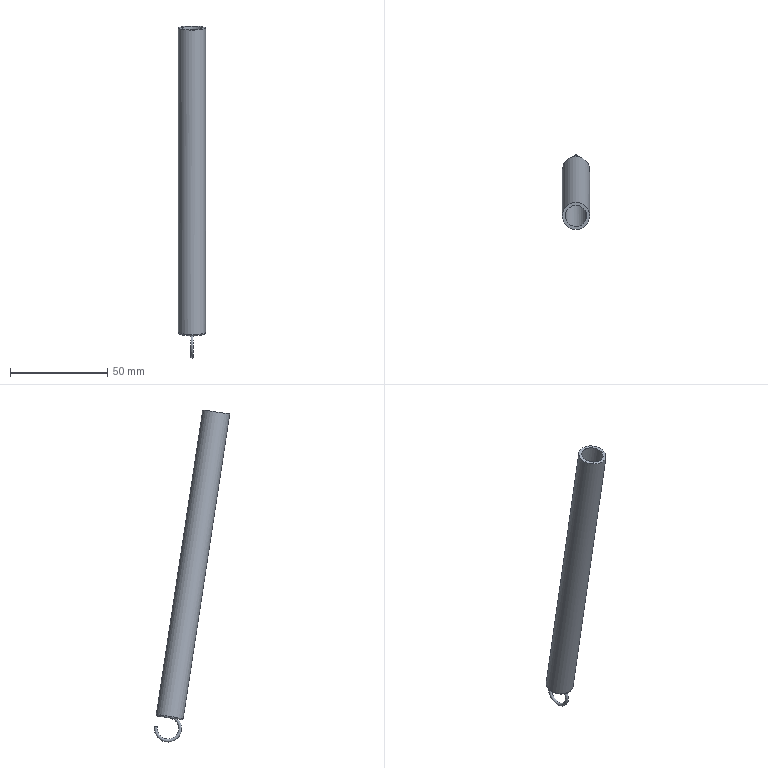Part | NX | features solid 2 | 1 solid | 7 faces | box 14 x 38.697 x 170.602 mm | volume 9414 mm3 | cylinder 3 | torus 2 | plane 2 | commonest cylinder face diameters 1.5 x1 11 x1 14 x1
STEP:
#1=CARTESIAN_POINT('',(-31.935,95.659,-933.338));
#2=VERTEX_POINT('',#1);
#3=CARTESIAN_POINT('',(-24.935,95.659,-933.338));
#4=DIRECTION('',(0.,-0.1507,0.9886));
#5=DIRECTION('',(-1.,0.,0.));
#6=AXIS2_PLACEMENT_3D('',#3,#4,#5);
#7=CIRCLE('',#6,7.);
#8=EDGE_CURVE('',#2,#2,#7,.T.);
#9=ORIENTED_EDGE('',*,*,#8,.T.);
#10=EDGE_LOOP('',(#9));
#11=FACE_BOUND('',#10,.T.);
#12=CARTESIAN_POINT('',(-24.935,78.749,-775.915));
#13=VERTEX_POINT('',#12);
#14=CARTESIAN_POINT('',(-24.935,71.827,-776.952));
#15=DIRECTION('',(0.,-0.1481,0.989));
#16=DIRECTION('',(0.,0.989,0.1481));
#17=AXIS2_PLACEMENT_3D('',#14,#15,#16);
#18=ELLIPSE('',#17,7.,7.);
#19=EDGE_CURVE('',#13,#13,#18,.F.);
#20=ORIENTED_EDGE('',*,*,#19,.T.);
#21=EDGE_LOOP('',(#20));
#22=FACE_BOUND('',#21,.T.);
#23=CARTESIAN_POINT('',(-24.935,59.467,-695.849));
#24=DIRECTION('',(0.,0.1507,-0.9886));
#25=DIRECTION('',(1.,0.,0.));
#26=AXIS2_PLACEMENT_3D('',#23,#24,#25);
#27=CYLINDRICAL_SURFACE('',#26,7.);
#28=ADVANCED_FACE('',(#11,#22),#27,.T.);
#29=CARTESIAN_POINT('',(-25.685,101.046,-932.517));
#30=VERTEX_POINT('',#29);
#31=CARTESIAN_POINT('',(-24.185,101.046,-932.517));
#32=VERTEX_POINT('',#31);
#33=CARTESIAN_POINT('',(-24.935,95.659,-933.338));
#34=DIRECTION('',(0.,-0.1507,0.9886));
#35=DIRECTION('',(1.,0.,0.));
#36=AXIS2_PLACEMENT_3D('',#33,#34,#35);
#37=CIRCLE('',#36,5.5);
#38=EDGE_CURVE('',#30,#32,#37,.T.);
#39=ORIENTED_EDGE('',*,*,#38,.F.);
#40=CARTESIAN_POINT('',(-24.185,101.046,-932.517));
#41=CARTESIAN_POINT('',(-24.185,100.986,-932.125));
#42=CARTESIAN_POINT('',(-24.934,100.981,-931.411));
#43=CARTESIAN_POINT('',(-25.685,100.986,-932.125));
#44=CARTESIAN_POINT('',(-25.685,101.046,-932.517));
#45=B_SPLINE_CURVE_WITH_KNOTS('',3,(#40,#41,#42,#43,#44),.UNSPECIFIED.,.F.,.F.,(4,1,4),(0.,0.001174,0.002347),.UNSPECIFIED.);
#46=EDGE_CURVE('',#32,#30,#45,.T.);
#47=ORIENTED_EDGE('',*,*,#46,.F.);
#48=EDGE_LOOP('',(#39,#47));
#49=FACE_BOUND('',#48,.T.);
#50=CARTESIAN_POINT('',(-24.935,77.266,-776.137));
#51=VERTEX_POINT('',#50);
#52=CARTESIAN_POINT('',(-24.935,71.827,-776.952));
#53=DIRECTION('',(0.,-0.1481,0.989));
#54=DIRECTION('',(0.,0.989,0.1481));
#55=AXIS2_PLACEMENT_3D('',#52,#53,#54);
#56=ELLIPSE('',#55,5.5,5.5);
#57=EDGE_CURVE('',#51,#51,#56,.T.);
#58=ORIENTED_EDGE('',*,*,#57,.T.);
#59=EDGE_LOOP('',(#58));
#60=FACE_BOUND('',#59,.T.);
#61=CARTESIAN_POINT('',(-24.935,59.467,-695.849));
#62=DIRECTION('',(0.,0.1507,-0.9886));
#63=DIRECTION('',(1.,0.,0.));
#64=AXIS2_PLACEMENT_3D('',#61,#62,#63);
#65=CYLINDRICAL_SURFACE('',#64,5.5);
#66=ADVANCED_FACE('',(#49,#60),#65,.F.);
#67=ORIENTED_EDGE('',*,*,#38,.T.);
#68=CARTESIAN_POINT('',(-24.935,101.951,-933.138));
#69=VERTEX_POINT('',#68);
#70=CARTESIAN_POINT('',(-24.185,101.046,-932.517));
#71=CARTESIAN_POINT('',(-24.185,101.083,-932.761));
#72=CARTESIAN_POINT('',(-24.428,101.419,-933.116));
#73=CARTESIAN_POINT('',(-24.763,101.781,-933.164));
#74=CARTESIAN_POINT('',(-24.935,101.951,-933.138));
#75=B_SPLINE_CURVE_WITH_KNOTS('',3,(#70,#71,#72,#73,#74),.UNSPECIFIED.,.F.,.F.,(4,1,4),(0.,0.0007272,0.001454),.UNSPECIFIED.);
#76=EDGE_CURVE('',#32,#69,#75,.T.);
#77=ORIENTED_EDGE('',*,*,#76,.T.);
#78=CARTESIAN_POINT('',(-25.685,101.046,-932.517));
#79=CARTESIAN_POINT('',(-25.685,101.083,-932.761));
#80=CARTESIAN_POINT('',(-25.442,101.419,-933.116));
#81=CARTESIAN_POINT('',(-25.106,101.781,-933.164));
#82=CARTESIAN_POINT('',(-24.935,101.951,-933.138));
#83=B_SPLINE_CURVE_WITH_KNOTS('',3,(#78,#79,#80,#81,#82),.UNSPECIFIED.,.F.,.F.,(4,1,4),(0.,0.0007272,0.001454),.UNSPECIFIED.);
#84=EDGE_CURVE('',#69,#30,#83,.F.);
#85=ORIENTED_EDGE('',*,*,#84,.T.);
#86=EDGE_LOOP('',(#67,#77,#85));
#87=FACE_BOUND('',#86,.T.);
#88=ORIENTED_EDGE('',*,*,#8,.F.);
#89=EDGE_LOOP('',(#88));
#90=FACE_BOUND('',#89,.T.);
#91=CARTESIAN_POINT('',(-24.935,95.659,-933.338));
#92=DIRECTION('',(0.,-0.1507,0.9886));
#93=DIRECTION('',(1.,0.,0.));
#94=AXIS2_PLACEMENT_3D('',#91,#92,#93);
#95=TOROIDAL_SURFACE('',#94,6.25,0.75);
#96=ADVANCED_FACE('',(#87,#90),#95,.T.);
#97=CARTESIAN_POINT('',(-24.935,103.501,-938.342));
#98=VERTEX_POINT('',#97);
#99=CARTESIAN_POINT('',(-24.935,102.762,-938.468));
#100=DIRECTION('',(0.,0.1679,-0.9858));
#101=DIRECTION('',(0.,0.9858,0.1679));
#102=AXIS2_PLACEMENT_3D('',#99,#100,#101);
#103=CIRCLE('',#102,0.75);
#104=EDGE_CURVE('',#98,#98,#103,.T.);
#105=ORIENTED_EDGE('',*,*,#104,.T.);
#106=EDGE_LOOP('',(#105));
#107=FACE_BOUND('',#106,.T.);
#108=CARTESIAN_POINT('',(-25.685,95.659,-933.338));
#109=VERTEX_POINT('',#108);
#110=CARTESIAN_POINT('',(-24.935,95.659,-933.338));
#111=DIRECTION('',(0.,0.9886,0.1507));
#112=DIRECTION('',(-1.,0.,0.));
#113=AXIS2_PLACEMENT_3D('',#110,#111,#112);
#114=CIRCLE('',#113,0.75);
#115=EDGE_CURVE('',#109,#109,#114,.T.);
#116=ORIENTED_EDGE('',*,*,#115,.F.);
#117=EDGE_LOOP('',(#116));
#118=FACE_BOUND('',#117,.T.);
#119=CARTESIAN_POINT('',(-24.935,96.601,-939.517));
#120=DIRECTION('',(1.,0.,0.));
#121=DIRECTION('',(0.,0.1507,-0.9886));
#122=AXIS2_PLACEMENT_3D('',#119,#120,#121);
#123=TOROIDAL_SURFACE('',#122,6.25,0.75);
#124=ADVANCED_FACE('',(#107,#118),#123,.T.);
#125=ORIENTED_EDGE('',*,*,#115,.T.);
#126=EDGE_LOOP('',(#125));
#127=FACE_BOUND('',#126,.T.);
#128=ORIENTED_EDGE('',*,*,#76,.F.);
#129=ORIENTED_EDGE('',*,*,#46,.T.);
#130=ORIENTED_EDGE('',*,*,#84,.F.);
#131=EDGE_LOOP('',(#128,#129,#130));
#132=FACE_BOUND('',#131,.T.);
#133=CARTESIAN_POINT('',(-24.935,98.748,-932.867));
#134=DIRECTION('',(0.,-0.9886,-0.1507));
#135=DIRECTION('',(1.,0.,0.));
#136=AXIS2_PLACEMENT_3D('',#133,#134,#135);
#137=CYLINDRICAL_SURFACE('',#136,0.75);
#138=ADVANCED_FACE('',(#127,#132),#137,.T.);
#139=ORIENTED_EDGE('',*,*,#104,.F.);
#140=EDGE_LOOP('',(#139));
#141=FACE_BOUND('',#140,.T.);
#142=CARTESIAN_POINT('',(-24.935,102.762,-938.468));
#143=DIRECTION('',(0.,0.1679,-0.9858));
#144=DIRECTION('',(0.,-0.9858,-0.1679));
#145=AXIS2_PLACEMENT_3D('',#142,#143,#144);
#146=PLANE('',#145);
#147=ADVANCED_FACE('',(#141),#146,.F.);
#148=ORIENTED_EDGE('',*,*,#19,.F.);
#149=EDGE_LOOP('',(#148));
#150=FACE_BOUND('',#149,.T.);
#151=ORIENTED_EDGE('',*,*,#57,.F.);
#152=EDGE_LOOP('',(#151));
#153=FACE_BOUND('',#152,.T.);
#154=CARTESIAN_POINT('',(-80.065,113.799,-770.665));
#155=DIRECTION('',(0.,-0.1481,0.989));
#156=DIRECTION('',(0.,-0.989,-0.1481));
#157=AXIS2_PLACEMENT_3D('',#154,#155,#156);
#158=PLANE('',#157);
#159=ADVANCED_FACE('',(#150,#153),#158,.T.);
#160=CLOSED_SHELL('',(#28,#66,#96,#124,#138,#147,#159));
#161=MANIFOLD_SOLID_BREP('',#160);
#162=(LENGTH_UNIT()NAMED_UNIT(*)SI_UNIT(.MILLI.,.METRE.));
#163=UNCERTAINTY_MEASURE_WITH_UNIT(LENGTH_MEASURE(0.0508),#162,'','');
#164=(NAMED_UNIT(*)PLANE_ANGLE_UNIT()SI_UNIT($,.RADIAN.));
#165=(NAMED_UNIT(*)SI_UNIT($,.STERADIAN.)SOLID_ANGLE_UNIT());
#166=(GEOMETRIC_REPRESENTATION_CONTEXT(3)GLOBAL_UNCERTAINTY_ASSIGNED_CONTEXT((#163))GLOBAL_UNIT_ASSIGNED_CONTEXT((#162,#164,#165))REPRESENTATION_CONTEXT('',''));
#167=ADVANCED_BREP_SHAPE_REPRESENTATION('',(#161),#166);